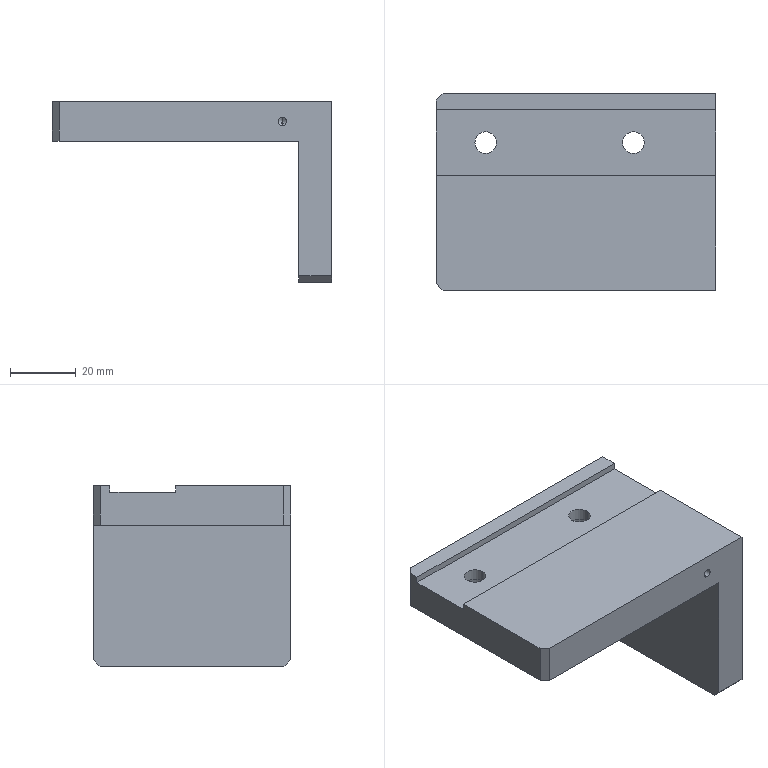Part | SolidWorks | features HoleWzd 5, ICE 4, Chamfer 2, Extrusion 1 | 1 solid | 38 faces | box 85 x 60 x 55 mm | volume 81319 mm3 | plane 18 | cylinder 14 | cone 6 | commonest cylinder face diameters 5 x4 6.6 x4 11 x4 2.5 x2
STEP:
#1=CARTESIAN_POINT('',(82.5,-15.,-26.));
#2=VERTEX_POINT('',#1);
#3=CARTESIAN_POINT('',(77.5,-15.,-26.));
#4=VERTEX_POINT('',#3);
#5=CARTESIAN_POINT('',(80.,-15.,-26.));
#6=DIRECTION('',(0.,0.,-1.));
#7=DIRECTION('',(-1.,0.,0.));
#8=AXIS2_PLACEMENT_3D('',#5,#6,#7);
#9=CIRCLE('',#8,2.5);
#10=EDGE_CURVE('',#2,#4,#9,.T.);
#11=ORIENTED_EDGE('',*,*,#10,.F.);
#12=CARTESIAN_POINT('',(82.5,-15.,-43.));
#13=VERTEX_POINT('',#12);
#14=CARTESIAN_POINT('',(82.5,-15.,-43.));
#15=DIRECTION('',(0.,0.,-1.));
#16=VECTOR('',#15,1000.);
#17=LINE('',#14,#16);
#18=EDGE_CURVE('',#2,#13,#17,.T.);
#19=ORIENTED_EDGE('',*,*,#18,.T.);
#20=CARTESIAN_POINT('',(77.5,-15.,-43.));
#21=VERTEX_POINT('',#20);
#22=CARTESIAN_POINT('',(80.,-15.,-43.));
#23=DIRECTION('',(0.,0.,-1.));
#24=DIRECTION('',(-1.,0.,0.));
#25=AXIS2_PLACEMENT_3D('',#22,#23,#24);
#26=CIRCLE('',#25,2.5);
#27=EDGE_CURVE('',#13,#21,#26,.T.);
#28=ORIENTED_EDGE('',*,*,#27,.T.);
#29=CARTESIAN_POINT('',(77.5,-15.,-43.));
#30=DIRECTION('',(0.,0.,-1.));
#31=VECTOR('',#30,1000.);
#32=LINE('',#29,#31);
#33=EDGE_CURVE('',#4,#21,#32,.T.);
#34=ORIENTED_EDGE('',*,*,#33,.F.);
#35=EDGE_LOOP('',(#11,#19,#28,#34));
#36=FACE_OUTER_BOUND('',#35,.T.);
#37=CARTESIAN_POINT('',(80.,-15.,-43.));
#38=DIRECTION('',(0.,0.,-1.));
#39=DIRECTION('',(-1.,0.,0.));
#40=AXIS2_PLACEMENT_3D('',#37,#38,#39);
#41=CYLINDRICAL_SURFACE('',#40,2.5);
#42=ADVANCED_FACE('',(#36),#41,.F.);
#43=CARTESIAN_POINT('',(80.,-15.,-24.498));
#44=VERTEX_POINT('',#43);
#45=CARTESIAN_POINT('',(77.5,-15.,-26.));
#46=DIRECTION('',(-0.8572,0.,-0.515));
#47=VECTOR('',#46,1000.);
#48=LINE('',#45,#47);
#49=EDGE_CURVE('',#44,#4,#48,.T.);
#50=ORIENTED_EDGE('',*,*,#49,.F.);
#51=CARTESIAN_POINT('',(82.5,-15.,-26.));
#52=DIRECTION('',(0.8572,0.,-0.515));
#53=VECTOR('',#52,1000.);
#54=LINE('',#51,#53);
#55=EDGE_CURVE('',#44,#2,#54,.T.);
#56=ORIENTED_EDGE('',*,*,#55,.T.);
#57=ORIENTED_EDGE('',*,*,#10,.T.);
#58=EDGE_LOOP('',(#50,#56,#57));
#59=FACE_OUTER_BOUND('',#58,.T.);
#60=CARTESIAN_POINT('',(80.,-15.,-26.));
#61=DIRECTION('',(0.,0.,-1.));
#62=DIRECTION('',(-1.,0.,0.));
#63=AXIS2_PLACEMENT_3D('',#60,#61,#62);
#64=CONICAL_SURFACE('',#63,2.5,1.03);
#65=ADVANCED_FACE('',(#59),#64,.F.);
#66=CARTESIAN_POINT('',(82.5,-45.,-26.));
#67=VERTEX_POINT('',#66);
#68=CARTESIAN_POINT('',(77.5,-45.,-26.));
#69=VERTEX_POINT('',#68);
#70=CARTESIAN_POINT('',(80.,-45.,-26.));
#71=DIRECTION('',(0.,0.,-1.));
#72=DIRECTION('',(-1.,0.,0.));
#73=AXIS2_PLACEMENT_3D('',#70,#71,#72);
#74=CIRCLE('',#73,2.5);
#75=EDGE_CURVE('',#67,#69,#74,.T.);
#76=ORIENTED_EDGE('',*,*,#75,.F.);
#77=CARTESIAN_POINT('',(82.5,-45.,-43.));
#78=VERTEX_POINT('',#77);
#79=CARTESIAN_POINT('',(82.5,-45.,-43.));
#80=DIRECTION('',(0.,0.,-1.));
#81=VECTOR('',#80,1000.);
#82=LINE('',#79,#81);
#83=EDGE_CURVE('',#67,#78,#82,.T.);
#84=ORIENTED_EDGE('',*,*,#83,.T.);
#85=CARTESIAN_POINT('',(77.5,-45.,-43.));
#86=VERTEX_POINT('',#85);
#87=CARTESIAN_POINT('',(80.,-45.,-43.));
#88=DIRECTION('',(0.,0.,-1.));
#89=DIRECTION('',(-1.,0.,0.));
#90=AXIS2_PLACEMENT_3D('',#87,#88,#89);
#91=CIRCLE('',#90,2.5);
#92=EDGE_CURVE('',#78,#86,#91,.T.);
#93=ORIENTED_EDGE('',*,*,#92,.T.);
#94=CARTESIAN_POINT('',(77.5,-45.,-43.));
#95=DIRECTION('',(0.,0.,-1.));
#96=VECTOR('',#95,1000.);
#97=LINE('',#94,#96);
#98=EDGE_CURVE('',#69,#86,#97,.T.);
#99=ORIENTED_EDGE('',*,*,#98,.F.);
#100=EDGE_LOOP('',(#76,#84,#93,#99));
#101=FACE_OUTER_BOUND('',#100,.T.);
#102=CARTESIAN_POINT('',(80.,-45.,-43.));
#103=DIRECTION('',(0.,0.,-1.));
#104=DIRECTION('',(-1.,0.,0.));
#105=AXIS2_PLACEMENT_3D('',#102,#103,#104);
#106=CYLINDRICAL_SURFACE('',#105,2.5);
#107=ADVANCED_FACE('',(#101),#106,.F.);
#108=CARTESIAN_POINT('',(80.,-45.,-24.498));
#109=VERTEX_POINT('',#108);
#110=CARTESIAN_POINT('',(77.5,-45.,-26.));
#111=DIRECTION('',(-0.8572,0.,-0.515));
#112=VECTOR('',#111,1000.);
#113=LINE('',#110,#112);
#114=EDGE_CURVE('',#109,#69,#113,.T.);
#115=ORIENTED_EDGE('',*,*,#114,.F.);
#116=CARTESIAN_POINT('',(82.5,-45.,-26.));
#117=DIRECTION('',(0.8572,0.,-0.515));
#118=VECTOR('',#117,1000.);
#119=LINE('',#116,#118);
#120=EDGE_CURVE('',#109,#67,#119,.T.);
#121=ORIENTED_EDGE('',*,*,#120,.T.);
#122=ORIENTED_EDGE('',*,*,#75,.T.);
#123=EDGE_LOOP('',(#115,#121,#122));
#124=FACE_OUTER_BOUND('',#123,.T.);
#125=CARTESIAN_POINT('',(80.,-45.,-26.));
#126=DIRECTION('',(0.,0.,-1.));
#127=DIRECTION('',(-1.,0.,0.));
#128=AXIS2_PLACEMENT_3D('',#125,#126,#127);
#129=CONICAL_SURFACE('',#128,2.5,1.03);
#130=ADVANCED_FACE('',(#124),#129,.F.);
#131=CARTESIAN_POINT('',(70.,-51.5,7.25));
#132=VERTEX_POINT('',#131);
#133=CARTESIAN_POINT('',(70.,-51.5,4.75));
#134=VERTEX_POINT('',#133);
#135=CARTESIAN_POINT('',(70.,-51.5,6.));
#136=DIRECTION('',(0.,-1.,0.));
#137=DIRECTION('',(0.,0.,-1.));
#138=AXIS2_PLACEMENT_3D('',#135,#136,#137);
#139=CIRCLE('',#138,1.25);
#140=EDGE_CURVE('',#132,#134,#139,.T.);
#141=ORIENTED_EDGE('',*,*,#140,.F.);
#142=CARTESIAN_POINT('',(70.,-60.,7.25));
#143=VERTEX_POINT('',#142);
#144=CARTESIAN_POINT('',(70.,-60.,7.25));
#145=DIRECTION('',(0.,-1.,0.));
#146=VECTOR('',#145,1000.);
#147=LINE('',#144,#146);
#148=EDGE_CURVE('',#132,#143,#147,.T.);
#149=ORIENTED_EDGE('',*,*,#148,.T.);
#150=CARTESIAN_POINT('',(70.,-60.,4.75));
#151=VERTEX_POINT('',#150);
#152=CARTESIAN_POINT('',(70.,-60.,6.));
#153=DIRECTION('',(0.,-1.,0.));
#154=DIRECTION('',(0.,0.,-1.));
#155=AXIS2_PLACEMENT_3D('',#152,#153,#154);
#156=CIRCLE('',#155,1.25);
#157=EDGE_CURVE('',#143,#151,#156,.T.);
#158=ORIENTED_EDGE('',*,*,#157,.T.);
#159=CARTESIAN_POINT('',(70.,-60.,4.75));
#160=DIRECTION('',(0.,-1.,0.));
#161=VECTOR('',#160,1000.);
#162=LINE('',#159,#161);
#163=EDGE_CURVE('',#134,#151,#162,.T.);
#164=ORIENTED_EDGE('',*,*,#163,.F.);
#165=EDGE_LOOP('',(#141,#149,#158,#164));
#166=FACE_OUTER_BOUND('',#165,.T.);
#167=CARTESIAN_POINT('',(70.,-60.,6.));
#168=DIRECTION('',(0.,-1.,0.));
#169=DIRECTION('',(0.,0.,-1.));
#170=AXIS2_PLACEMENT_3D('',#167,#168,#169);
#171=CYLINDRICAL_SURFACE('',#170,1.25);
#172=ADVANCED_FACE('',(#166),#171,.F.);
#173=CARTESIAN_POINT('',(70.,-50.749,6.));
#174=VERTEX_POINT('',#173);
#175=CARTESIAN_POINT('',(70.,-51.5,4.75));
#176=DIRECTION('',(0.,-0.515,-0.8572));
#177=VECTOR('',#176,1000.);
#178=LINE('',#175,#177);
#179=EDGE_CURVE('',#174,#134,#178,.T.);
#180=ORIENTED_EDGE('',*,*,#179,.F.);
#181=CARTESIAN_POINT('',(70.,-51.5,7.25));
#182=DIRECTION('',(0.,-0.515,0.8572));
#183=VECTOR('',#182,1000.);
#184=LINE('',#181,#183);
#185=EDGE_CURVE('',#174,#132,#184,.T.);
#186=ORIENTED_EDGE('',*,*,#185,.T.);
#187=ORIENTED_EDGE('',*,*,#140,.T.);
#188=EDGE_LOOP('',(#180,#186,#187));
#189=FACE_OUTER_BOUND('',#188,.T.);
#190=CARTESIAN_POINT('',(70.,-51.5,6.));
#191=DIRECTION('',(0.,-1.,0.));
#192=DIRECTION('',(0.,0.,-1.));
#193=AXIS2_PLACEMENT_3D('',#190,#191,#192);
#194=CONICAL_SURFACE('',#193,1.25,1.03);
#195=ADVANCED_FACE('',(#189),#194,.F.);
#196=CARTESIAN_POINT('',(65.5,-15.,6.4));
#197=VERTEX_POINT('',#196);
#198=CARTESIAN_POINT('',(54.5,-15.,6.4));
#199=VERTEX_POINT('',#198);
#200=CARTESIAN_POINT('',(60.,-15.,6.4));
#201=DIRECTION('',(0.,0.,-1.));
#202=DIRECTION('',(-1.,0.,0.));
#203=AXIS2_PLACEMENT_3D('',#200,#201,#202);
#204=CIRCLE('',#203,5.5);
#205=EDGE_CURVE('',#197,#199,#204,.T.);
#206=ORIENTED_EDGE('',*,*,#205,.F.);
#207=CARTESIAN_POINT('',(65.5,-15.,0.));
#208=VERTEX_POINT('',#207);
#209=CARTESIAN_POINT('',(65.5,-15.,0.));
#210=DIRECTION('',(0.,0.,-1.));
#211=VECTOR('',#210,1000.);
#212=LINE('',#209,#211);
#213=EDGE_CURVE('',#197,#208,#212,.T.);
#214=ORIENTED_EDGE('',*,*,#213,.T.);
#215=CARTESIAN_POINT('',(54.5,-15.,0.));
#216=VERTEX_POINT('',#215);
#217=CARTESIAN_POINT('',(60.,-15.,0.));
#218=DIRECTION('',(0.,0.,-1.));
#219=DIRECTION('',(-1.,0.,0.));
#220=AXIS2_PLACEMENT_3D('',#217,#218,#219);
#221=CIRCLE('',#220,5.5);
#222=EDGE_CURVE('',#208,#216,#221,.T.);
#223=ORIENTED_EDGE('',*,*,#222,.T.);
#224=CARTESIAN_POINT('',(54.5,-15.,0.));
#225=DIRECTION('',(0.,0.,-1.));
#226=VECTOR('',#225,1000.);
#227=LINE('',#224,#226);
#228=EDGE_CURVE('',#199,#216,#227,.T.);
#229=ORIENTED_EDGE('',*,*,#228,.F.);
#230=EDGE_LOOP('',(#206,#214,#223,#229));
#231=FACE_OUTER_BOUND('',#230,.T.);
#232=CARTESIAN_POINT('',(60.,-15.,0.));
#233=DIRECTION('',(0.,0.,-1.));
#234=DIRECTION('',(-1.,0.,0.));
#235=AXIS2_PLACEMENT_3D('',#232,#233,#234);
#236=CYLINDRICAL_SURFACE('',#235,5.5);
#237=ADVANCED_FACE('',(#231),#236,.F.);
#238=CARTESIAN_POINT('',(63.3,-15.,10.));
#239=VERTEX_POINT('',#238);
#240=CARTESIAN_POINT('',(56.7,-15.,10.));
#241=VERTEX_POINT('',#240);
#242=CARTESIAN_POINT('',(60.,-15.,10.));
#243=DIRECTION('',(0.,0.,-1.));
#244=DIRECTION('',(0.,1.,0.));
#245=AXIS2_PLACEMENT_3D('',#242,#243,#244);
#246=CIRCLE('',#245,3.3);
#247=EDGE_CURVE('',#239,#241,#246,.T.);
#248=ORIENTED_EDGE('',*,*,#247,.F.);
#249=CARTESIAN_POINT('',(63.3,-15.,6.4));
#250=VERTEX_POINT('',#249);
#251=CARTESIAN_POINT('',(63.3,-15.,0.));
#252=DIRECTION('',(0.,0.,-1.));
#253=VECTOR('',#252,1000.);
#254=LINE('',#251,#253);
#255=EDGE_CURVE('',#239,#250,#254,.T.);
#256=ORIENTED_EDGE('',*,*,#255,.T.);
#257=CARTESIAN_POINT('',(56.7,-15.,6.4));
#258=VERTEX_POINT('',#257);
#259=CARTESIAN_POINT('',(60.,-15.,6.4));
#260=DIRECTION('',(0.,0.,-1.));
#261=DIRECTION('',(-1.,0.,0.));
#262=AXIS2_PLACEMENT_3D('',#259,#260,#261);
#263=CIRCLE('',#262,3.3);
#264=EDGE_CURVE('',#250,#258,#263,.T.);
#265=ORIENTED_EDGE('',*,*,#264,.T.);
#266=CARTESIAN_POINT('',(56.7,-15.,0.));
#267=DIRECTION('',(0.,0.,-1.));
#268=VECTOR('',#267,1000.);
#269=LINE('',#266,#268);
#270=EDGE_CURVE('',#241,#258,#269,.T.);
#271=ORIENTED_EDGE('',*,*,#270,.F.);
#272=EDGE_LOOP('',(#248,#256,#265,#271));
#273=FACE_OUTER_BOUND('',#272,.T.);
#274=CARTESIAN_POINT('',(60.,-15.,0.));
#275=DIRECTION('',(0.,0.,-1.));
#276=DIRECTION('',(-1.,0.,0.));
#277=AXIS2_PLACEMENT_3D('',#274,#275,#276);
#278=CYLINDRICAL_SURFACE('',#277,3.3);
#279=ADVANCED_FACE('',(#273),#278,.F.);
#280=CARTESIAN_POINT('',(20.5,-15.,6.4));
#281=VERTEX_POINT('',#280);
#282=CARTESIAN_POINT('',(9.5,-15.,6.4));
#283=VERTEX_POINT('',#282);
#284=CARTESIAN_POINT('',(15.,-15.,6.4));
#285=DIRECTION('',(0.,0.,-1.));
#286=DIRECTION('',(-1.,0.,0.));
#287=AXIS2_PLACEMENT_3D('',#284,#285,#286);
#288=CIRCLE('',#287,5.5);
#289=EDGE_CURVE('',#281,#283,#288,.T.);
#290=ORIENTED_EDGE('',*,*,#289,.F.);
#291=CARTESIAN_POINT('',(20.5,-15.,0.));
#292=VERTEX_POINT('',#291);
#293=CARTESIAN_POINT('',(20.5,-15.,0.));
#294=DIRECTION('',(0.,0.,-1.));
#295=VECTOR('',#294,1000.);
#296=LINE('',#293,#295);
#297=EDGE_CURVE('',#281,#292,#296,.T.);
#298=ORIENTED_EDGE('',*,*,#297,.T.);
#299=CARTESIAN_POINT('',(9.5,-15.,0.));
#300=VERTEX_POINT('',#299);
#301=CARTESIAN_POINT('',(15.,-15.,0.));
#302=DIRECTION('',(0.,0.,-1.));
#303=DIRECTION('',(-1.,0.,0.));
#304=AXIS2_PLACEMENT_3D('',#301,#302,#303);
#305=CIRCLE('',#304,5.5);
#306=EDGE_CURVE('',#292,#300,#305,.T.);
#307=ORIENTED_EDGE('',*,*,#306,.T.);
#308=CARTESIAN_POINT('',(9.5,-15.,0.));
#309=DIRECTION('',(0.,0.,-1.));
#310=VECTOR('',#309,1000.);
#311=LINE('',#308,#310);
#312=EDGE_CURVE('',#283,#300,#311,.T.);
#313=ORIENTED_EDGE('',*,*,#312,.F.);
#314=EDGE_LOOP('',(#290,#298,#307,#313));
#315=FACE_OUTER_BOUND('',#314,.T.);
#316=CARTESIAN_POINT('',(15.,-15.,0.));
#317=DIRECTION('',(0.,0.,-1.));
#318=DIRECTION('',(-1.,0.,0.));
#319=AXIS2_PLACEMENT_3D('',#316,#317,#318);
#320=CYLINDRICAL_SURFACE('',#319,5.5);
#321=ADVANCED_FACE('',(#315),#320,.F.);
#322=CARTESIAN_POINT('',(18.3,-15.,10.));
#323=VERTEX_POINT('',#322);
#324=CARTESIAN_POINT('',(11.7,-15.,10.));
#325=VERTEX_POINT('',#324);
#326=CARTESIAN_POINT('',(15.,-15.,10.));
#327=DIRECTION('',(0.,0.,-1.));
#328=DIRECTION('',(0.,1.,0.));
#329=AXIS2_PLACEMENT_3D('',#326,#327,#328);
#330=CIRCLE('',#329,3.3);
#331=EDGE_CURVE('',#323,#325,#330,.T.);
#332=ORIENTED_EDGE('',*,*,#331,.F.);
#333=CARTESIAN_POINT('',(18.3,-15.,6.4));
#334=VERTEX_POINT('',#333);
#335=CARTESIAN_POINT('',(18.3,-15.,0.));
#336=DIRECTION('',(0.,0.,-1.));
#337=VECTOR('',#336,1000.);
#338=LINE('',#335,#337);
#339=EDGE_CURVE('',#323,#334,#338,.T.);
#340=ORIENTED_EDGE('',*,*,#339,.T.);
#341=CARTESIAN_POINT('',(11.7,-15.,6.4));
#342=VERTEX_POINT('',#341);
#343=CARTESIAN_POINT('',(15.,-15.,6.4));
#344=DIRECTION('',(0.,0.,-1.));
#345=DIRECTION('',(-1.,0.,0.));
#346=AXIS2_PLACEMENT_3D('',#343,#344,#345);
#347=CIRCLE('',#346,3.3);
#348=EDGE_CURVE('',#334,#342,#347,.T.);
#349=ORIENTED_EDGE('',*,*,#348,.T.);
#350=CARTESIAN_POINT('',(11.7,-15.,0.));
#351=DIRECTION('',(0.,0.,-1.));
#352=VECTOR('',#351,1000.);
#353=LINE('',#350,#352);
#354=EDGE_CURVE('',#325,#342,#353,.T.);
#355=ORIENTED_EDGE('',*,*,#354,.F.);
#356=EDGE_LOOP('',(#332,#340,#349,#355));
#357=FACE_OUTER_BOUND('',#356,.T.);
#358=CARTESIAN_POINT('',(15.,-15.,0.));
#359=DIRECTION('',(0.,0.,-1.));
#360=DIRECTION('',(-1.,0.,0.));
#361=AXIS2_PLACEMENT_3D('',#358,#359,#360);
#362=CYLINDRICAL_SURFACE('',#361,3.3);
#363=ADVANCED_FACE('',(#357),#362,.F.);
#364=CARTESIAN_POINT('',(60.,-15.,0.));
#365=DIRECTION('',(0.,0.,-1.));
#366=DIRECTION('',(-1.,0.,0.));
#367=AXIS2_PLACEMENT_3D('',#364,#365,#366);
#368=CIRCLE('',#367,5.5);
#369=EDGE_CURVE('',#216,#208,#368,.T.);
#370=ORIENTED_EDGE('',*,*,#369,.F.);
#371=ORIENTED_EDGE('',*,*,#222,.F.);
#372=EDGE_LOOP('',(#370,#371));
#373=FACE_BOUND('',#372,.T.);
#374=CARTESIAN_POINT('',(15.,-15.,0.));
#375=DIRECTION('',(0.,0.,-1.));
#376=DIRECTION('',(-1.,0.,0.));
#377=AXIS2_PLACEMENT_3D('',#374,#375,#376);
#378=CIRCLE('',#377,5.5);
#379=EDGE_CURVE('',#300,#292,#378,.T.);
#380=ORIENTED_EDGE('',*,*,#379,.F.);
#381=ORIENTED_EDGE('',*,*,#306,.F.);
#382=EDGE_LOOP('',(#380,#381));
#383=FACE_BOUND('',#382,.T.);
#384=CARTESIAN_POINT('',(2.,-60.,0.));
#385=VERTEX_POINT('',#384);
#386=CARTESIAN_POINT('',(75.,-60.,0.));
#387=VERTEX_POINT('',#386);
#388=CARTESIAN_POINT('',(0.,-60.,0.));
#389=DIRECTION('',(1.,0.,0.));
#390=VECTOR('',#389,1000.);
#391=LINE('',#388,#390);
#392=EDGE_CURVE('',#385,#387,#391,.T.);
#393=ORIENTED_EDGE('',*,*,#392,.F.);
#394=CARTESIAN_POINT('',(0.,-58.,0.));
#395=VERTEX_POINT('',#394);
#396=CARTESIAN_POINT('',(2.,-60.,0.));
#397=DIRECTION('',(-0.7071,0.7071,0.));
#398=VECTOR('',#397,1000.);
#399=LINE('',#396,#398);
#400=EDGE_CURVE('',#385,#395,#399,.T.);
#401=ORIENTED_EDGE('',*,*,#400,.T.);
#402=CARTESIAN_POINT('',(0.,-2.,0.));
#403=VERTEX_POINT('',#402);
#404=CARTESIAN_POINT('',(0.,0.,0.));
#405=DIRECTION('',(0.,-1.,0.));
#406=VECTOR('',#405,1000.);
#407=LINE('',#404,#406);
#408=EDGE_CURVE('',#403,#395,#407,.T.);
#409=ORIENTED_EDGE('',*,*,#408,.F.);
#410=CARTESIAN_POINT('',(2.,0.,0.));
#411=VERTEX_POINT('',#410);
#412=CARTESIAN_POINT('',(0.,-2.,0.));
#413=DIRECTION('',(0.7071,0.7071,0.));
#414=VECTOR('',#413,1000.);
#415=LINE('',#412,#414);
#416=EDGE_CURVE('',#403,#411,#415,.T.);
#417=ORIENTED_EDGE('',*,*,#416,.T.);
#418=CARTESIAN_POINT('',(75.,0.,0.));
#419=VERTEX_POINT('',#418);
#420=CARTESIAN_POINT('',(0.,0.,0.));
#421=DIRECTION('',(-1.,0.,0.));
#422=VECTOR('',#421,1000.);
#423=LINE('',#420,#422);
#424=EDGE_CURVE('',#419,#411,#423,.T.);
#425=ORIENTED_EDGE('',*,*,#424,.F.);
#426=CARTESIAN_POINT('',(75.,-60.,0.));
#427=DIRECTION('',(0.,1.,0.));
#428=VECTOR('',#427,1000.);
#429=LINE('',#426,#428);
#430=EDGE_CURVE('',#387,#419,#429,.T.);
#431=ORIENTED_EDGE('',*,*,#430,.F.);
#432=EDGE_LOOP('',(#393,#401,#409,#417,#425,#431));
#433=FACE_OUTER_BOUND('',#432,.T.);
#434=CARTESIAN_POINT('',(0.,0.,0.));
#435=DIRECTION('',(0.,0.,1.));
#436=DIRECTION('',(1.,0.,0.));
#437=AXIS2_PLACEMENT_3D('',#434,#435,#436);
#438=PLANE('',#437);
#439=ADVANCED_FACE('',(#373,#383,#433),#438,.F.);
#440=CARTESIAN_POINT('',(85.,-5.,12.));
#441=VERTEX_POINT('',#440);
#442=CARTESIAN_POINT('',(85.,0.,12.));
#443=VERTEX_POINT('',#442);
#444=CARTESIAN_POINT('',(85.,-60.,12.));
#445=DIRECTION('',(0.,1.,0.));
#446=VECTOR('',#445,1000.);
#447=LINE('',#444,#446);
#448=EDGE_CURVE('',#441,#443,#447,.T.);
#449=ORIENTED_EDGE('',*,*,#448,.T.);
#450=CARTESIAN_POINT('',(2.,0.,12.));
#451=VERTEX_POINT('',#450);
#452=CARTESIAN_POINT('',(0.,0.,12.));
#453=DIRECTION('',(-1.,0.,0.));
#454=VECTOR('',#453,1000.);
#455=LINE('',#452,#454);
#456=EDGE_CURVE('',#443,#451,#455,.T.);
#457=ORIENTED_EDGE('',*,*,#456,.T.);
#458=CARTESIAN_POINT('',(0.,-2.,12.));
#459=VERTEX_POINT('',#458);
#460=CARTESIAN_POINT('',(1.,-1.,12.));
#461=DIRECTION('',(-0.7071,-0.7071,0.));
#462=VECTOR('',#461,1000.);
#463=LINE('',#460,#462);
#464=EDGE_CURVE('',#451,#459,#463,.T.);
#465=ORIENTED_EDGE('',*,*,#464,.T.);
#466=CARTESIAN_POINT('',(0.,-5.,12.));
#467=VERTEX_POINT('',#466);
#468=CARTESIAN_POINT('',(0.,0.,12.));
#469=DIRECTION('',(0.,-1.,0.));
#470=VECTOR('',#469,1000.);
#471=LINE('',#468,#470);
#472=EDGE_CURVE('',#459,#467,#471,.T.);
#473=ORIENTED_EDGE('',*,*,#472,.T.);
#474=CARTESIAN_POINT('',(0.,-5.,12.));
#475=DIRECTION('',(1.,0.,0.));
#476=VECTOR('',#475,1000.);
#477=LINE('',#474,#476);
#478=EDGE_CURVE('',#467,#441,#477,.T.);
#479=ORIENTED_EDGE('',*,*,#478,.T.);
#480=EDGE_LOOP('',(#449,#457,#465,#473,#479));
#481=FACE_OUTER_BOUND('',#480,.T.);
#482=CARTESIAN_POINT('',(0.,0.,12.));
#483=DIRECTION('',(0.,0.,1.));
#484=DIRECTION('',(1.,0.,0.));
#485=AXIS2_PLACEMENT_3D('',#482,#483,#484);
#486=PLANE('',#485);
#487=ADVANCED_FACE('',(#481),#486,.T.);
#488=ORIENTED_EDGE('',*,*,#408,.T.);
#489=CARTESIAN_POINT('',(0.,-58.,12.));
#490=VERTEX_POINT('',#489);
#491=CARTESIAN_POINT('',(0.,-58.,12.));
#492=DIRECTION('',(0.,0.,1.));
#493=VECTOR('',#492,1000.);
#494=LINE('',#491,#493);
#495=EDGE_CURVE('',#395,#490,#494,.T.);
#496=ORIENTED_EDGE('',*,*,#495,.T.);
#497=CARTESIAN_POINT('',(0.,-25.,12.));
#498=VERTEX_POINT('',#497);
#499=CARTESIAN_POINT('',(0.,0.,12.));
#500=DIRECTION('',(0.,-1.,0.));
#501=VECTOR('',#500,1000.);
#502=LINE('',#499,#501);
#503=EDGE_CURVE('',#498,#490,#502,.T.);
#504=ORIENTED_EDGE('',*,*,#503,.F.);
#505=CARTESIAN_POINT('',(0.,-25.,10.));
#506=VERTEX_POINT('',#505);
#507=CARTESIAN_POINT('',(0.,-25.,12.));
#508=DIRECTION('',(0.,0.,-1.));
#509=VECTOR('',#508,1000.);
#510=LINE('',#507,#509);
#511=EDGE_CURVE('',#498,#506,#510,.T.);
#512=ORIENTED_EDGE('',*,*,#511,.T.);
#513=CARTESIAN_POINT('',(0.,-5.,10.));
#514=VERTEX_POINT('',#513);
#515=CARTESIAN_POINT('',(0.,-5.,10.));
#516=DIRECTION('',(0.,1.,0.));
#517=VECTOR('',#516,1000.);
#518=LINE('',#515,#517);
#519=EDGE_CURVE('',#506,#514,#518,.T.);
#520=ORIENTED_EDGE('',*,*,#519,.T.);
#521=CARTESIAN_POINT('',(0.,-5.,12.));
#522=DIRECTION('',(0.,0.,1.));
#523=VECTOR('',#522,1000.);
#524=LINE('',#521,#523);
#525=EDGE_CURVE('',#514,#467,#524,.T.);
#526=ORIENTED_EDGE('',*,*,#525,.T.);
#527=ORIENTED_EDGE('',*,*,#472,.F.);
#528=CARTESIAN_POINT('',(0.,-2.,12.));
#529=DIRECTION('',(0.,0.,-1.));
#530=VECTOR('',#529,1000.);
#531=LINE('',#528,#530);
#532=EDGE_CURVE('',#459,#403,#531,.T.);
#533=ORIENTED_EDGE('',*,*,#532,.T.);
#534=EDGE_LOOP('',(#488,#496,#504,#512,#520,#526,#527,#533));
#535=FACE_OUTER_BOUND('',#534,.T.);
#536=CARTESIAN_POINT('',(0.,0.,12.));
#537=DIRECTION('',(1.,0.,0.));
#538=DIRECTION('',(0.,1.,0.));
#539=AXIS2_PLACEMENT_3D('',#536,#537,#538);
#540=PLANE('',#539);
#541=ADVANCED_FACE('',(#535),#540,.F.);
#542=CARTESIAN_POINT('',(75.,-60.,-41.));
#543=VERTEX_POINT('',#542);
#544=CARTESIAN_POINT('',(75.,-60.,-43.));
#545=DIRECTION('',(0.,0.,1.));
#546=VECTOR('',#545,1000.);
#547=LINE('',#544,#546);
#548=EDGE_CURVE('',#543,#387,#547,.T.);
#549=ORIENTED_EDGE('',*,*,#548,.F.);
#550=CARTESIAN_POINT('',(85.,-60.,-41.));
#551=VERTEX_POINT('',#550);
#552=CARTESIAN_POINT('',(85.,-60.,-41.));
#553=DIRECTION('',(1.,0.,0.));
#554=VECTOR('',#553,1000.);
#555=LINE('',#552,#554);
#556=EDGE_CURVE('',#543,#551,#555,.T.);
#557=ORIENTED_EDGE('',*,*,#556,.T.);
#558=CARTESIAN_POINT('',(85.,-60.,12.));
#559=VERTEX_POINT('',#558);
#560=CARTESIAN_POINT('',(85.,-60.,-43.));
#561=DIRECTION('',(0.,0.,1.));
#562=VECTOR('',#561,1000.);
#563=LINE('',#560,#562);
#564=EDGE_CURVE('',#551,#559,#563,.T.);
#565=ORIENTED_EDGE('',*,*,#564,.T.);
#566=CARTESIAN_POINT('',(2.,-60.,12.));
#567=VERTEX_POINT('',#566);
#568=CARTESIAN_POINT('',(0.,-60.,12.));
#569=DIRECTION('',(1.,0.,0.));
#570=VECTOR('',#569,1000.);
#571=LINE('',#568,#570);
#572=EDGE_CURVE('',#567,#559,#571,.T.);
#573=ORIENTED_EDGE('',*,*,#572,.F.);
#574=CARTESIAN_POINT('',(2.,-60.,12.));
#575=DIRECTION('',(0.,0.,-1.));
#576=VECTOR('',#575,1000.);
#577=LINE('',#574,#576);
#578=EDGE_CURVE('',#567,#385,#577,.T.);
#579=ORIENTED_EDGE('',*,*,#578,.T.);
#580=ORIENTED_EDGE('',*,*,#392,.T.);
#581=EDGE_LOOP('',(#549,#557,#565,#573,#579,#580));
#582=FACE_OUTER_BOUND('',#581,.T.);
#583=CARTESIAN_POINT('',(70.,-60.,6.));
#584=DIRECTION('',(0.,-1.,0.));
#585=DIRECTION('',(0.,0.,-1.));
#586=AXIS2_PLACEMENT_3D('',#583,#584,#585);
#587=CIRCLE('',#586,1.25);
#588=EDGE_CURVE('',#151,#143,#587,.T.);
#589=ORIENTED_EDGE('',*,*,#588,.F.);
#590=ORIENTED_EDGE('',*,*,#157,.F.);
#591=EDGE_LOOP('',(#589,#590));
#592=FACE_BOUND('',#591,.T.);
#593=CARTESIAN_POINT('',(0.,-60.,12.));
#594=DIRECTION('',(0.,1.,0.));
#595=DIRECTION('',(0.,0.,1.));
#596=AXIS2_PLACEMENT_3D('',#593,#594,#595);
#597=PLANE('',#596);
#598=ADVANCED_FACE('',(#582,#592),#597,.F.);
#599=CARTESIAN_POINT('',(85.,0.,-41.));
#600=VERTEX_POINT('',#599);
#601=CARTESIAN_POINT('',(85.,0.,-43.));
#602=DIRECTION('',(0.,0.,1.));
#603=VECTOR('',#602,1000.);
#604=LINE('',#601,#603);
#605=EDGE_CURVE('',#600,#443,#604,.T.);
#606=ORIENTED_EDGE('',*,*,#605,.F.);
#607=CARTESIAN_POINT('',(75.,0.,-41.));
#608=VERTEX_POINT('',#607);
#609=CARTESIAN_POINT('',(75.,0.,-41.));
#610=DIRECTION('',(-1.,0.,0.));
#611=VECTOR('',#610,1000.);
#612=LINE('',#609,#611);
#613=EDGE_CURVE('',#600,#608,#612,.T.);
#614=ORIENTED_EDGE('',*,*,#613,.T.);
#615=CARTESIAN_POINT('',(75.,0.,-43.));
#616=DIRECTION('',(0.,0.,1.));
#617=VECTOR('',#616,1000.);
#618=LINE('',#615,#617);
#619=EDGE_CURVE('',#608,#419,#618,.T.);
#620=ORIENTED_EDGE('',*,*,#619,.T.);
#621=ORIENTED_EDGE('',*,*,#424,.T.);
#622=CARTESIAN_POINT('',(2.,0.,12.));
#623=DIRECTION('',(0.,0.,1.));
#624=VECTOR('',#623,1000.);
#625=LINE('',#622,#624);
#626=EDGE_CURVE('',#411,#451,#625,.T.);
#627=ORIENTED_EDGE('',*,*,#626,.T.);
#628=ORIENTED_EDGE('',*,*,#456,.F.);
#629=EDGE_LOOP('',(#606,#614,#620,#621,#627,#628));
#630=FACE_OUTER_BOUND('',#629,.T.);
#631=CARTESIAN_POINT('',(0.,0.,12.));
#632=DIRECTION('',(0.,-1.,0.));
#633=DIRECTION('',(0.,0.,-1.));
#634=AXIS2_PLACEMENT_3D('',#631,#632,#633);
#635=PLANE('',#634);
#636=ADVANCED_FACE('',(#630),#635,.F.);
#637=CARTESIAN_POINT('',(85.,-25.,12.));
#638=VERTEX_POINT('',#637);
#639=CARTESIAN_POINT('',(85.,-60.,12.));
#640=DIRECTION('',(0.,1.,0.));
#641=VECTOR('',#640,1000.);
#642=LINE('',#639,#641);
#643=EDGE_CURVE('',#559,#638,#642,.T.);
#644=ORIENTED_EDGE('',*,*,#643,.T.);
#645=CARTESIAN_POINT('',(0.,-25.,12.));
#646=DIRECTION('',(1.,0.,0.));
#647=VECTOR('',#646,1000.);
#648=LINE('',#645,#647);
#649=EDGE_CURVE('',#498,#638,#648,.T.);
#650=ORIENTED_EDGE('',*,*,#649,.F.);
#651=ORIENTED_EDGE('',*,*,#503,.T.);
#652=CARTESIAN_POINT('',(-29.,-29.,12.));
#653=DIRECTION('',(0.7071,-0.7071,0.));
#654=VECTOR('',#653,1000.);
#655=LINE('',#652,#654);
#656=EDGE_CURVE('',#490,#567,#655,.T.);
#657=ORIENTED_EDGE('',*,*,#656,.T.);
#658=ORIENTED_EDGE('',*,*,#572,.T.);
#659=EDGE_LOOP('',(#644,#650,#651,#657,#658));
#660=FACE_OUTER_BOUND('',#659,.T.);
#661=CARTESIAN_POINT('',(0.,0.,12.));
#662=DIRECTION('',(0.,0.,1.));
#663=DIRECTION('',(1.,0.,0.));
#664=AXIS2_PLACEMENT_3D('',#661,#662,#663);
#665=PLANE('',#664);
#666=ADVANCED_FACE('',(#660),#665,.T.);
#667=CARTESIAN_POINT('',(85.,-5.,10.));
#668=VERTEX_POINT('',#667);
#669=CARTESIAN_POINT('',(0.,-5.,10.));
#670=DIRECTION('',(1.,0.,0.));
#671=VECTOR('',#670,1000.);
#672=LINE('',#669,#671);
#673=EDGE_CURVE('',#514,#668,#672,.T.);
#674=ORIENTED_EDGE('',*,*,#673,.T.);
#675=CARTESIAN_POINT('',(85.,-5.,12.));
#676=DIRECTION('',(0.,0.,1.));
#677=VECTOR('',#676,1000.);
#678=LINE('',#675,#677);
#679=EDGE_CURVE('',#668,#441,#678,.T.);
#680=ORIENTED_EDGE('',*,*,#679,.T.);
#681=ORIENTED_EDGE('',*,*,#478,.F.);
#682=ORIENTED_EDGE('',*,*,#525,.F.);
#683=EDGE_LOOP('',(#674,#680,#681,#682));
#684=FACE_OUTER_BOUND('',#683,.T.);
#685=CARTESIAN_POINT('',(0.,-5.,12.));
#686=DIRECTION('',(0.,1.,0.));
#687=DIRECTION('',(0.,0.,1.));
#688=AXIS2_PLACEMENT_3D('',#685,#686,#687);
#689=PLANE('',#688);
#690=ADVANCED_FACE('',(#684),#689,.F.);
#691=CARTESIAN_POINT('',(60.,-15.,10.));
#692=DIRECTION('',(0.,0.,-1.));
#693=DIRECTION('',(0.,1.,0.));
#694=AXIS2_PLACEMENT_3D('',#691,#692,#693);
#695=CIRCLE('',#694,3.3);
#696=EDGE_CURVE('',#241,#239,#695,.T.);
#697=ORIENTED_EDGE('',*,*,#696,.T.);
#698=ORIENTED_EDGE('',*,*,#247,.T.);
#699=EDGE_LOOP('',(#697,#698));
#700=FACE_BOUND('',#699,.T.);
#701=CARTESIAN_POINT('',(15.,-15.,10.));
#702=DIRECTION('',(0.,0.,-1.));
#703=DIRECTION('',(0.,1.,0.));
#704=AXIS2_PLACEMENT_3D('',#701,#702,#703);
#705=CIRCLE('',#704,3.3);
#706=EDGE_CURVE('',#325,#323,#705,.T.);
#707=ORIENTED_EDGE('',*,*,#706,.T.);
#708=ORIENTED_EDGE('',*,*,#331,.T.);
#709=EDGE_LOOP('',(#707,#708));
#710=FACE_BOUND('',#709,.T.);
#711=CARTESIAN_POINT('',(85.,-25.,10.));
#712=VERTEX_POINT('',#711);
#713=CARTESIAN_POINT('',(0.,-25.,10.));
#714=DIRECTION('',(1.,0.,0.));
#715=VECTOR('',#714,1000.);
#716=LINE('',#713,#715);
#717=EDGE_CURVE('',#506,#712,#716,.T.);
#718=ORIENTED_EDGE('',*,*,#717,.T.);
#719=CARTESIAN_POINT('',(85.,-5.,10.));
#720=DIRECTION('',(0.,1.,0.));
#721=VECTOR('',#720,1000.);
#722=LINE('',#719,#721);
#723=EDGE_CURVE('',#712,#668,#722,.T.);
#724=ORIENTED_EDGE('',*,*,#723,.T.);
#725=ORIENTED_EDGE('',*,*,#673,.F.);
#726=ORIENTED_EDGE('',*,*,#519,.F.);
#727=EDGE_LOOP('',(#718,#724,#725,#726));
#728=FACE_OUTER_BOUND('',#727,.T.);
#729=CARTESIAN_POINT('',(0.,-5.,10.));
#730=DIRECTION('',(0.,0.,-1.));
#731=DIRECTION('',(0.,1.,0.));
#732=AXIS2_PLACEMENT_3D('',#729,#730,#731);
#733=PLANE('',#732);
#734=ADVANCED_FACE('',(#700,#710,#728),#733,.F.);
#735=ORIENTED_EDGE('',*,*,#649,.T.);
#736=CARTESIAN_POINT('',(85.,-25.,12.));
#737=DIRECTION('',(0.,0.,-1.));
#738=VECTOR('',#737,1000.);
#739=LINE('',#736,#738);
#740=EDGE_CURVE('',#638,#712,#739,.T.);
#741=ORIENTED_EDGE('',*,*,#740,.T.);
#742=ORIENTED_EDGE('',*,*,#717,.F.);
#743=ORIENTED_EDGE('',*,*,#511,.F.);
#744=EDGE_LOOP('',(#735,#741,#742,#743));
#745=FACE_OUTER_BOUND('',#744,.T.);
#746=CARTESIAN_POINT('',(0.,-25.,12.));
#747=DIRECTION('',(0.,-1.,0.));
#748=DIRECTION('',(1.,0.,0.));
#749=AXIS2_PLACEMENT_3D('',#746,#747,#748);
#750=PLANE('',#749);
#751=ADVANCED_FACE('',(#745),#750,.F.);
#752=ORIENTED_EDGE('',*,*,#339,.F.);
#753=ORIENTED_EDGE('',*,*,#706,.F.);
#754=ORIENTED_EDGE('',*,*,#354,.T.);
#755=CARTESIAN_POINT('',(15.,-15.,6.4));
#756=DIRECTION('',(0.,0.,-1.));
#757=DIRECTION('',(-1.,0.,0.));
#758=AXIS2_PLACEMENT_3D('',#755,#756,#757);
#759=CIRCLE('',#758,3.3);
#760=EDGE_CURVE('',#342,#334,#759,.T.);
#761=ORIENTED_EDGE('',*,*,#760,.T.);
#762=EDGE_LOOP('',(#752,#753,#754,#761));
#763=FACE_OUTER_BOUND('',#762,.T.);
#764=CARTESIAN_POINT('',(15.,-15.,0.));
#765=DIRECTION('',(0.,0.,-1.));
#766=DIRECTION('',(-1.,0.,0.));
#767=AXIS2_PLACEMENT_3D('',#764,#765,#766);
#768=CYLINDRICAL_SURFACE('',#767,3.3);
#769=ADVANCED_FACE('',(#763),#768,.F.);
#770=ORIENTED_EDGE('',*,*,#760,.F.);
#771=ORIENTED_EDGE('',*,*,#348,.F.);
#772=EDGE_LOOP('',(#770,#771));
#773=FACE_BOUND('',#772,.T.);
#774=CARTESIAN_POINT('',(15.,-15.,6.4));
#775=DIRECTION('',(0.,0.,-1.));
#776=DIRECTION('',(-1.,0.,0.));
#777=AXIS2_PLACEMENT_3D('',#774,#775,#776);
#778=CIRCLE('',#777,5.5);
#779=EDGE_CURVE('',#283,#281,#778,.T.);
#780=ORIENTED_EDGE('',*,*,#779,.T.);
#781=ORIENTED_EDGE('',*,*,#289,.T.);
#782=EDGE_LOOP('',(#780,#781));
#783=FACE_OUTER_BOUND('',#782,.T.);
#784=CARTESIAN_POINT('',(18.3,-15.,6.4));
#785=DIRECTION('',(0.,0.,1.));
#786=DIRECTION('',(1.,0.,0.));
#787=AXIS2_PLACEMENT_3D('',#784,#785,#786);
#788=PLANE('',#787);
#789=ADVANCED_FACE('',(#773,#783),#788,.F.);
#790=ORIENTED_EDGE('',*,*,#297,.F.);
#791=ORIENTED_EDGE('',*,*,#779,.F.);
#792=ORIENTED_EDGE('',*,*,#312,.T.);
#793=ORIENTED_EDGE('',*,*,#379,.T.);
#794=EDGE_LOOP('',(#790,#791,#792,#793));
#795=FACE_OUTER_BOUND('',#794,.T.);
#796=CARTESIAN_POINT('',(15.,-15.,0.));
#797=DIRECTION('',(0.,0.,-1.));
#798=DIRECTION('',(-1.,0.,0.));
#799=AXIS2_PLACEMENT_3D('',#796,#797,#798);
#800=CYLINDRICAL_SURFACE('',#799,5.5);
#801=ADVANCED_FACE('',(#795),#800,.F.);
#802=ORIENTED_EDGE('',*,*,#255,.F.);
#803=ORIENTED_EDGE('',*,*,#696,.F.);
#804=ORIENTED_EDGE('',*,*,#270,.T.);
#805=CARTESIAN_POINT('',(60.,-15.,6.4));
#806=DIRECTION('',(0.,0.,-1.));
#807=DIRECTION('',(-1.,0.,0.));
#808=AXIS2_PLACEMENT_3D('',#805,#806,#807);
#809=CIRCLE('',#808,3.3);
#810=EDGE_CURVE('',#258,#250,#809,.T.);
#811=ORIENTED_EDGE('',*,*,#810,.T.);
#812=EDGE_LOOP('',(#802,#803,#804,#811));
#813=FACE_OUTER_BOUND('',#812,.T.);
#814=CARTESIAN_POINT('',(60.,-15.,0.));
#815=DIRECTION('',(0.,0.,-1.));
#816=DIRECTION('',(-1.,0.,0.));
#817=AXIS2_PLACEMENT_3D('',#814,#815,#816);
#818=CYLINDRICAL_SURFACE('',#817,3.3);
#819=ADVANCED_FACE('',(#813),#818,.F.);
#820=ORIENTED_EDGE('',*,*,#810,.F.);
#821=ORIENTED_EDGE('',*,*,#264,.F.);
#822=EDGE_LOOP('',(#820,#821));
#823=FACE_BOUND('',#822,.T.);
#824=CARTESIAN_POINT('',(60.,-15.,6.4));
#825=DIRECTION('',(0.,0.,-1.));
#826=DIRECTION('',(-1.,0.,0.));
#827=AXIS2_PLACEMENT_3D('',#824,#825,#826);
#828=CIRCLE('',#827,5.5);
#829=EDGE_CURVE('',#199,#197,#828,.T.);
#830=ORIENTED_EDGE('',*,*,#829,.T.);
#831=ORIENTED_EDGE('',*,*,#205,.T.);
#832=EDGE_LOOP('',(#830,#831));
#833=FACE_OUTER_BOUND('',#832,.T.);
#834=CARTESIAN_POINT('',(63.3,-15.,6.4));
#835=DIRECTION('',(0.,0.,1.));
#836=DIRECTION('',(1.,0.,0.));
#837=AXIS2_PLACEMENT_3D('',#834,#835,#836);
#838=PLANE('',#837);
#839=ADVANCED_FACE('',(#823,#833),#838,.F.);
#840=ORIENTED_EDGE('',*,*,#213,.F.);
#841=ORIENTED_EDGE('',*,*,#829,.F.);
#842=ORIENTED_EDGE('',*,*,#228,.T.);
#843=ORIENTED_EDGE('',*,*,#369,.T.);
#844=EDGE_LOOP('',(#840,#841,#842,#843));
#845=FACE_OUTER_BOUND('',#844,.T.);
#846=CARTESIAN_POINT('',(60.,-15.,0.));
#847=DIRECTION('',(0.,0.,-1.));
#848=DIRECTION('',(-1.,0.,0.));
#849=AXIS2_PLACEMENT_3D('',#846,#847,#848);
#850=CYLINDRICAL_SURFACE('',#849,5.5);
#851=ADVANCED_FACE('',(#845),#850,.F.);
#852=ORIENTED_EDGE('',*,*,#656,.F.);
#853=ORIENTED_EDGE('',*,*,#495,.F.);
#854=ORIENTED_EDGE('',*,*,#400,.F.);
#855=ORIENTED_EDGE('',*,*,#578,.F.);
#856=EDGE_LOOP('',(#852,#853,#854,#855));
#857=FACE_OUTER_BOUND('',#856,.T.);
#858=CARTESIAN_POINT('',(2.,-60.,12.));
#859=DIRECTION('',(0.7071,0.7071,0.));
#860=DIRECTION('',(0.,0.,-1.));
#861=AXIS2_PLACEMENT_3D('',#858,#859,#860);
#862=PLANE('',#861);
#863=ADVANCED_FACE('',(#857),#862,.F.);
#864=ORIENTED_EDGE('',*,*,#464,.F.);
#865=ORIENTED_EDGE('',*,*,#626,.F.);
#866=ORIENTED_EDGE('',*,*,#416,.F.);
#867=ORIENTED_EDGE('',*,*,#532,.F.);
#868=EDGE_LOOP('',(#864,#865,#866,#867));
#869=FACE_OUTER_BOUND('',#868,.T.);
#870=CARTESIAN_POINT('',(0.,-2.,12.));
#871=DIRECTION('',(0.7071,-0.7071,0.));
#872=DIRECTION('',(0.,0.,-1.));
#873=AXIS2_PLACEMENT_3D('',#870,#871,#872);
#874=PLANE('',#873);
#875=ADVANCED_FACE('',(#869),#874,.F.);
#876=ORIENTED_EDGE('',*,*,#185,.F.);
#877=ORIENTED_EDGE('',*,*,#179,.T.);
#878=CARTESIAN_POINT('',(70.,-51.5,6.));
#879=DIRECTION('',(0.,-1.,0.));
#880=DIRECTION('',(0.,0.,-1.));
#881=AXIS2_PLACEMENT_3D('',#878,#879,#880);
#882=CIRCLE('',#881,1.25);
#883=EDGE_CURVE('',#134,#132,#882,.T.);
#884=ORIENTED_EDGE('',*,*,#883,.T.);
#885=EDGE_LOOP('',(#876,#877,#884));
#886=FACE_OUTER_BOUND('',#885,.T.);
#887=CARTESIAN_POINT('',(70.,-51.5,6.));
#888=DIRECTION('',(0.,-1.,0.));
#889=DIRECTION('',(0.,0.,-1.));
#890=AXIS2_PLACEMENT_3D('',#887,#888,#889);
#891=CONICAL_SURFACE('',#890,1.25,1.03);
#892=ADVANCED_FACE('',(#886),#891,.F.);
#893=ORIENTED_EDGE('',*,*,#148,.F.);
#894=ORIENTED_EDGE('',*,*,#883,.F.);
#895=ORIENTED_EDGE('',*,*,#163,.T.);
#896=ORIENTED_EDGE('',*,*,#588,.T.);
#897=EDGE_LOOP('',(#893,#894,#895,#896));
#898=FACE_OUTER_BOUND('',#897,.T.);
#899=CARTESIAN_POINT('',(70.,-60.,6.));
#900=DIRECTION('',(0.,-1.,0.));
#901=DIRECTION('',(0.,0.,-1.));
#902=AXIS2_PLACEMENT_3D('',#899,#900,#901);
#903=CYLINDRICAL_SURFACE('',#902,1.25);
#904=ADVANCED_FACE('',(#898),#903,.F.);
#905=CARTESIAN_POINT('',(85.,-2.,-43.));
#906=VERTEX_POINT('',#905);
#907=CARTESIAN_POINT('',(85.,-58.,-43.));
#908=VERTEX_POINT('',#907);
#909=CARTESIAN_POINT('',(85.,0.,-43.));
#910=DIRECTION('',(0.,-1.,0.));
#911=VECTOR('',#910,1000.);
#912=LINE('',#909,#911);
#913=EDGE_CURVE('',#906,#908,#912,.T.);
#914=ORIENTED_EDGE('',*,*,#913,.F.);
#915=CARTESIAN_POINT('',(85.,-2.,-43.));
#916=DIRECTION('',(0.,0.7071,0.7071));
#917=VECTOR('',#916,1000.);
#918=LINE('',#915,#917);
#919=EDGE_CURVE('',#906,#600,#918,.T.);
#920=ORIENTED_EDGE('',*,*,#919,.T.);
#921=ORIENTED_EDGE('',*,*,#605,.T.);
#922=ORIENTED_EDGE('',*,*,#448,.F.);
#923=ORIENTED_EDGE('',*,*,#679,.F.);
#924=ORIENTED_EDGE('',*,*,#723,.F.);
#925=ORIENTED_EDGE('',*,*,#740,.F.);
#926=ORIENTED_EDGE('',*,*,#643,.F.);
#927=ORIENTED_EDGE('',*,*,#564,.F.);
#928=CARTESIAN_POINT('',(85.,-58.,-43.));
#929=DIRECTION('',(0.,0.7071,-0.7071));
#930=VECTOR('',#929,1000.);
#931=LINE('',#928,#930);
#932=EDGE_CURVE('',#551,#908,#931,.T.);
#933=ORIENTED_EDGE('',*,*,#932,.T.);
#934=EDGE_LOOP('',(#914,#920,#921,#922,#923,#924,#925,#926,#927,#933));
#935=FACE_OUTER_BOUND('',#934,.T.);
#936=CARTESIAN_POINT('',(85.,0.,-43.));
#937=DIRECTION('',(-1.,0.,0.));
#938=DIRECTION('',(0.,0.,1.));
#939=AXIS2_PLACEMENT_3D('',#936,#937,#938);
#940=PLANE('',#939);
#941=ADVANCED_FACE('',(#935),#940,.F.);
#942=ORIENTED_EDGE('',*,*,#619,.F.);
#943=CARTESIAN_POINT('',(75.,-2.,-43.));
#944=VERTEX_POINT('',#943);
#945=CARTESIAN_POINT('',(75.,-2.,-43.));
#946=DIRECTION('',(0.,-0.7071,-0.7071));
#947=VECTOR('',#946,1000.);
#948=LINE('',#945,#947);
#949=EDGE_CURVE('',#608,#944,#948,.T.);
#950=ORIENTED_EDGE('',*,*,#949,.T.);
#951=CARTESIAN_POINT('',(75.,-58.,-43.));
#952=VERTEX_POINT('',#951);
#953=CARTESIAN_POINT('',(75.,0.,-43.));
#954=DIRECTION('',(0.,1.,0.));
#955=VECTOR('',#954,1000.);
#956=LINE('',#953,#955);
#957=EDGE_CURVE('',#952,#944,#956,.T.);
#958=ORIENTED_EDGE('',*,*,#957,.F.);
#959=CARTESIAN_POINT('',(75.,-58.,-43.));
#960=DIRECTION('',(0.,-0.7071,0.7071));
#961=VECTOR('',#960,1000.);
#962=LINE('',#959,#961);
#963=EDGE_CURVE('',#952,#543,#962,.T.);
#964=ORIENTED_EDGE('',*,*,#963,.T.);
#965=ORIENTED_EDGE('',*,*,#548,.T.);
#966=ORIENTED_EDGE('',*,*,#430,.T.);
#967=EDGE_LOOP('',(#942,#950,#958,#964,#965,#966));
#968=FACE_OUTER_BOUND('',#967,.T.);
#969=CARTESIAN_POINT('',(75.,0.,-43.));
#970=DIRECTION('',(1.,0.,0.));
#971=DIRECTION('',(0.,0.,-1.));
#972=AXIS2_PLACEMENT_3D('',#969,#970,#971);
#973=PLANE('',#972);
#974=ADVANCED_FACE('',(#968),#973,.F.);
#975=CARTESIAN_POINT('',(80.,-15.,-43.));
#976=DIRECTION('',(0.,0.,-1.));
#977=DIRECTION('',(-1.,0.,0.));
#978=AXIS2_PLACEMENT_3D('',#975,#976,#977);
#979=CIRCLE('',#978,2.5);
#980=EDGE_CURVE('',#21,#13,#979,.T.);
#981=ORIENTED_EDGE('',*,*,#980,.F.);
#982=ORIENTED_EDGE('',*,*,#27,.F.);
#983=EDGE_LOOP('',(#981,#982));
#984=FACE_BOUND('',#983,.T.);
#985=CARTESIAN_POINT('',(80.,-45.,-43.));
#986=DIRECTION('',(0.,0.,-1.));
#987=DIRECTION('',(-1.,0.,0.));
#988=AXIS2_PLACEMENT_3D('',#985,#986,#987);
#989=CIRCLE('',#988,2.5);
#990=EDGE_CURVE('',#86,#78,#989,.T.);
#991=ORIENTED_EDGE('',*,*,#990,.F.);
#992=ORIENTED_EDGE('',*,*,#92,.F.);
#993=EDGE_LOOP('',(#991,#992));
#994=FACE_BOUND('',#993,.T.);
#995=ORIENTED_EDGE('',*,*,#957,.T.);
#996=CARTESIAN_POINT('',(85.,-2.,-43.));
#997=DIRECTION('',(1.,0.,0.));
#998=VECTOR('',#997,1000.);
#999=LINE('',#996,#998);
#1000=EDGE_CURVE('',#944,#906,#999,.T.);
#1001=ORIENTED_EDGE('',*,*,#1000,.T.);
#1002=ORIENTED_EDGE('',*,*,#913,.T.);
#1003=CARTESIAN_POINT('',(75.,-58.,-43.));
#1004=DIRECTION('',(-1.,0.,0.));
#1005=VECTOR('',#1004,1000.);
#1006=LINE('',#1003,#1005);
#1007=EDGE_CURVE('',#908,#952,#1006,.T.);
#1008=ORIENTED_EDGE('',*,*,#1007,.T.);
#1009=EDGE_LOOP('',(#995,#1001,#1002,#1008));
#1010=FACE_OUTER_BOUND('',#1009,.T.);
#1011=CARTESIAN_POINT('',(0.,0.,-43.));
#1012=DIRECTION('',(0.,0.,-1.));
#1013=DIRECTION('',(-1.,0.,0.));
#1014=AXIS2_PLACEMENT_3D('',#1011,#1012,#1013);
#1015=PLANE('',#1014);
#1016=ADVANCED_FACE('',(#984,#994,#1010),#1015,.T.);
#1017=ORIENTED_EDGE('',*,*,#120,.F.);
#1018=ORIENTED_EDGE('',*,*,#114,.T.);
#1019=CARTESIAN_POINT('',(80.,-45.,-26.));
#1020=DIRECTION('',(0.,0.,-1.));
#1021=DIRECTION('',(-1.,0.,0.));
#1022=AXIS2_PLACEMENT_3D('',#1019,#1020,#1021);
#1023=CIRCLE('',#1022,2.5);
#1024=EDGE_CURVE('',#69,#67,#1023,.T.);
#1025=ORIENTED_EDGE('',*,*,#1024,.T.);
#1026=EDGE_LOOP('',(#1017,#1018,#1025));
#1027=FACE_OUTER_BOUND('',#1026,.T.);
#1028=CARTESIAN_POINT('',(80.,-45.,-26.));
#1029=DIRECTION('',(0.,0.,-1.));
#1030=DIRECTION('',(-1.,0.,0.));
#1031=AXIS2_PLACEMENT_3D('',#1028,#1029,#1030);
#1032=CONICAL_SURFACE('',#1031,2.5,1.03);
#1033=ADVANCED_FACE('',(#1027),#1032,.F.);
#1034=ORIENTED_EDGE('',*,*,#83,.F.);
#1035=ORIENTED_EDGE('',*,*,#1024,.F.);
#1036=ORIENTED_EDGE('',*,*,#98,.T.);
#1037=ORIENTED_EDGE('',*,*,#990,.T.);
#1038=EDGE_LOOP('',(#1034,#1035,#1036,#1037));
#1039=FACE_OUTER_BOUND('',#1038,.T.);
#1040=CARTESIAN_POINT('',(80.,-45.,-43.));
#1041=DIRECTION('',(0.,0.,-1.));
#1042=DIRECTION('',(-1.,0.,0.));
#1043=AXIS2_PLACEMENT_3D('',#1040,#1041,#1042);
#1044=CYLINDRICAL_SURFACE('',#1043,2.5);
#1045=ADVANCED_FACE('',(#1039),#1044,.F.);
#1046=ORIENTED_EDGE('',*,*,#55,.F.);
#1047=ORIENTED_EDGE('',*,*,#49,.T.);
#1048=CARTESIAN_POINT('',(80.,-15.,-26.));
#1049=DIRECTION('',(0.,0.,-1.));
#1050=DIRECTION('',(-1.,0.,0.));
#1051=AXIS2_PLACEMENT_3D('',#1048,#1049,#1050);
#1052=CIRCLE('',#1051,2.5);
#1053=EDGE_CURVE('',#4,#2,#1052,.T.);
#1054=ORIENTED_EDGE('',*,*,#1053,.T.);
#1055=EDGE_LOOP('',(#1046,#1047,#1054));
#1056=FACE_OUTER_BOUND('',#1055,.T.);
#1057=CARTESIAN_POINT('',(80.,-15.,-26.));
#1058=DIRECTION('',(0.,0.,-1.));
#1059=DIRECTION('',(-1.,0.,0.));
#1060=AXIS2_PLACEMENT_3D('',#1057,#1058,#1059);
#1061=CONICAL_SURFACE('',#1060,2.5,1.03);
#1062=ADVANCED_FACE('',(#1056),#1061,.F.);
#1063=ORIENTED_EDGE('',*,*,#18,.F.);
#1064=ORIENTED_EDGE('',*,*,#1053,.F.);
#1065=ORIENTED_EDGE('',*,*,#33,.T.);
#1066=ORIENTED_EDGE('',*,*,#980,.T.);
#1067=EDGE_LOOP('',(#1063,#1064,#1065,#1066));
#1068=FACE_OUTER_BOUND('',#1067,.T.);
#1069=CARTESIAN_POINT('',(80.,-15.,-43.));
#1070=DIRECTION('',(0.,0.,-1.));
#1071=DIRECTION('',(-1.,0.,0.));
#1072=AXIS2_PLACEMENT_3D('',#1069,#1070,#1071);
#1073=CYLINDRICAL_SURFACE('',#1072,2.5);
#1074=ADVANCED_FACE('',(#1068),#1073,.F.);
#1075=ORIENTED_EDGE('',*,*,#949,.F.);
#1076=ORIENTED_EDGE('',*,*,#613,.F.);
#1077=ORIENTED_EDGE('',*,*,#919,.F.);
#1078=ORIENTED_EDGE('',*,*,#1000,.F.);
#1079=EDGE_LOOP('',(#1075,#1076,#1077,#1078));
#1080=FACE_OUTER_BOUND('',#1079,.T.);
#1081=CARTESIAN_POINT('',(0.,-2.,-43.));
#1082=DIRECTION('',(0.,0.7071,-0.7071));
#1083=DIRECTION('',(-1.,0.,0.));
#1084=AXIS2_PLACEMENT_3D('',#1081,#1082,#1083);
#1085=PLANE('',#1084);
#1086=ADVANCED_FACE('',(#1080),#1085,.T.);
#1087=ORIENTED_EDGE('',*,*,#932,.F.);
#1088=ORIENTED_EDGE('',*,*,#556,.F.);
#1089=ORIENTED_EDGE('',*,*,#963,.F.);
#1090=ORIENTED_EDGE('',*,*,#1007,.F.);
#1091=EDGE_LOOP('',(#1087,#1088,#1089,#1090));
#1092=FACE_OUTER_BOUND('',#1091,.T.);
#1093=CARTESIAN_POINT('',(0.,-58.,-43.));
#1094=DIRECTION('',(0.,-0.7071,-0.7071));
#1095=DIRECTION('',(1.,0.,0.));
#1096=AXIS2_PLACEMENT_3D('',#1093,#1094,#1095);
#1097=PLANE('',#1096);
#1098=ADVANCED_FACE('',(#1092),#1097,.T.);
#1099=CLOSED_SHELL('',(#42,#65,#107,#130,#172,#195,#237,#279,#321,#363,#439,#487,#541,#598,#636,#666,#690,#734,#751,#769,#789,#801,#819,#839,#851,#863,#875,#892,#904,#941,#974,#1016,#1033,#1045,#1062,#1074,#1086,#1098));
#1100=MANIFOLD_SOLID_BREP('',#1099);
#1101=CARTESIAN_POINT('',(0.,0.,0.));
#1102=DIRECTION('',(0.,0.,1.));
#1103=DIRECTION('',(1.,0.,0.));
#1104=AXIS2_PLACEMENT_3D('',#1101,#1102,#1103);
#1105=(LENGTH_UNIT()NAMED_UNIT(*)SI_UNIT(.MILLI.,.METRE.));
#1106=UNCERTAINTY_MEASURE_WITH_UNIT(LENGTH_MEASURE(0.00001),#1105,'','');
#1107=(NAMED_UNIT(*)PLANE_ANGLE_UNIT()SI_UNIT($,.RADIAN.));
#1108=(NAMED_UNIT(*)SI_UNIT($,.STERADIAN.)SOLID_ANGLE_UNIT());
#1109=(GEOMETRIC_REPRESENTATION_CONTEXT(3)GLOBAL_UNCERTAINTY_ASSIGNED_CONTEXT((#1106))GLOBAL_UNIT_ASSIGNED_CONTEXT((#1105,#1107,#1108))REPRESENTATION_CONTEXT('',''));
#1110=ADVANCED_BREP_SHAPE_REPRESENTATION('',(#1100,#1104),#1109);